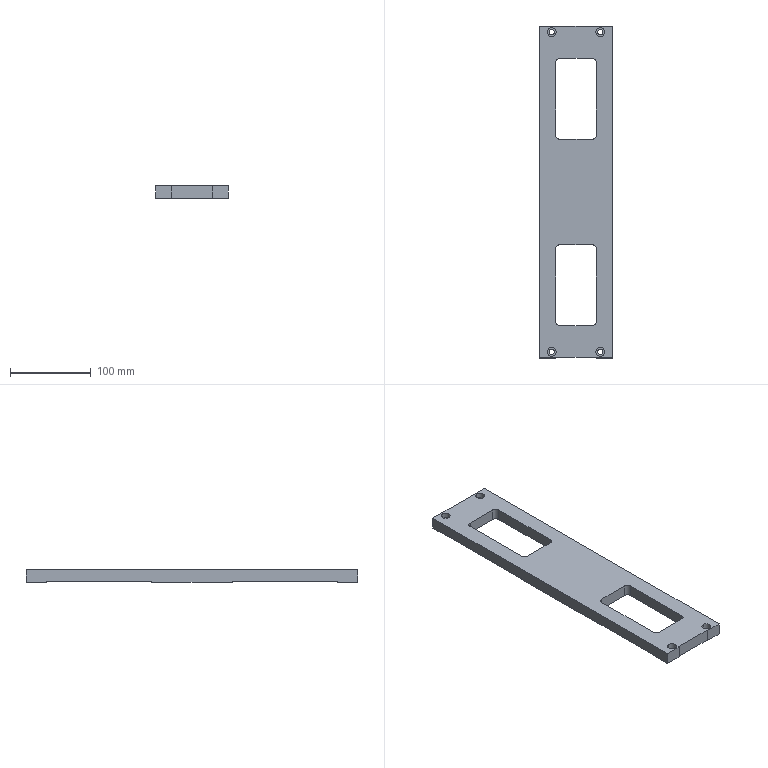CAM job | NX | 3-axis milling, drilling | part box 90 x 410 x 15 mm | stock box 94 x 414 x 15 mm
Tools:
number,name,description,diameter,corner_radius,flute_length,length,flutes
7,D6A45,Milling Tool-5 Parameters,6.0,0.0,50.0,75.0,2
16,6.6ZT,Drilling Tool,6.6,0.0,35.0,50.0,2
13,3.3ZT,Drilling Tool,3.3,0.0,35.0,50.0,2
3,D3,Milling Tool-5 Parameters,3.0,0.0,50.0,75.0,2
4,D4,Milling Tool-5 Parameters,4.0,0.0,50.0,75.0,2
10,D10,Milling Tool-5 Parameters,10.0,0.0,50.0,75.0,2
11,D10JING,Milling Tool-5 Parameters,10.0,0.0,50.0,75.0,2
6,D6,Milling Tool-5 Parameters,6.0,0.0,50.0,75.0,2
Operations:
program,operation,operation_type,tool,method,geometry_group,spindle_rpm,surface_speed,feed_per_tooth,feed_cut,feed_plunge,cut_length_mm,path_length_mm,cut_time_min,machine_time_min
1,DRILLING,Operation,D6A45,METHOD,A,5000.0,94.0,0.025,250.0,0.0,56.0,857.236,0.224,0.3041
1,DRILLING_COPY,Operation,6.6ZT,METHOD,A,2000.0,28.0,0.05,200.0,0.0,79.931,744.024,0.3997,0.4661
1,DRILLING_COPY_COPY,Operation,3.3ZT,METHOD,A,2000.0,28.0,0.05,200.0,0.0,56.366,358.97,0.2818,0.3121
1,ZLEVEL_PROFILE,ZLevelMilling,D10,METHOD,A,9500.0,298.0,0.1579,3000.0,1000.0,51676.866,51748.816,17.248,17.256
1,PLANAR_MILL,PlanarMilling,D10,METHOD,A,9500.0,298.0,0.1579,3000.0,1000.0,78660.732,81590.302,27.494,27.787
1,FLOOR_WALL,VolumeBased25DMillingOperation,D10,METHOD,A,9500.0,298.0,0.1316,2500.0,1000.0,9812.091,10271.333,3.948,3.994
1,CAVITY_MILL_COPY_1,CavityMilling,D10JING,METHOD,A,9500.0,298.0,0.0632,1200.0,1000.0,1039.189,1127.089,0.8666,0.8754
1,CAVITY_MILL_COPY_1_COPY,CavityMilling,D10JING,METHOD,A,9500.0,298.0,0.0632,1200.0,1000.0,537.261,1030.791,0.4492,0.4985
1,FLOOR_WALL_COPY,VolumeBased25DMillingOperation,D10,METHOD,A,9500.0,298.0,0.0632,1200.0,1000.0,5685.972,6470.987,4.742,4.821
1,HOLE_MILLING,CylinderMilling,D4,METHOD,A,9500.0,119.0,0.0789,1500.0,100.0,401.871,932.871,0.2679,0.321
1,HOLE_MILLING_COPY,CylinderMilling,D3,METHOD,A,9500.0,89.0,0.0632,1200.0,100.0,277.75,705.291,0.2315,0.2742
1,PLANAR_MILL_1,PlanarMilling,D6A45,METHOD,A,9500.0,179.0,0.0658,1250.0,100.0,740.789,3014.73,0.5926,0.82
1,PLANAR_MILL_1_COPY,PlanarMilling,D6A45,METHOD,A,9500.0,179.0,0.0658,1250.0,100.0,1124.226,2138.497,0.8994,1.001
1,刀补4,CylinderMilling,D4,METHOD,A,9500.0,119.0,0.0789,1500.0,100.0,71.457,602.457,0.0476,0.1007
1,刀补3,CylinderMilling,D3,METHOD,A,9500.0,89.0,0.0632,1200.0,100.0,61.927,489.468,0.0516,0.0944
2,HOLE_MILLING_1,CylinderMilling,D6,METHOD,B,9500.0,179.0,0.0737,1400.0,100.0,1024.63,1809.761,0.7319,0.8104
2,PLANAR_MILL_1_COPY_COPY,PlanarMilling,D6A45,METHOD,B,9500.0,179.0,0.0658,1250.0,100.0,1743.78,2691.706,1.395,1.49